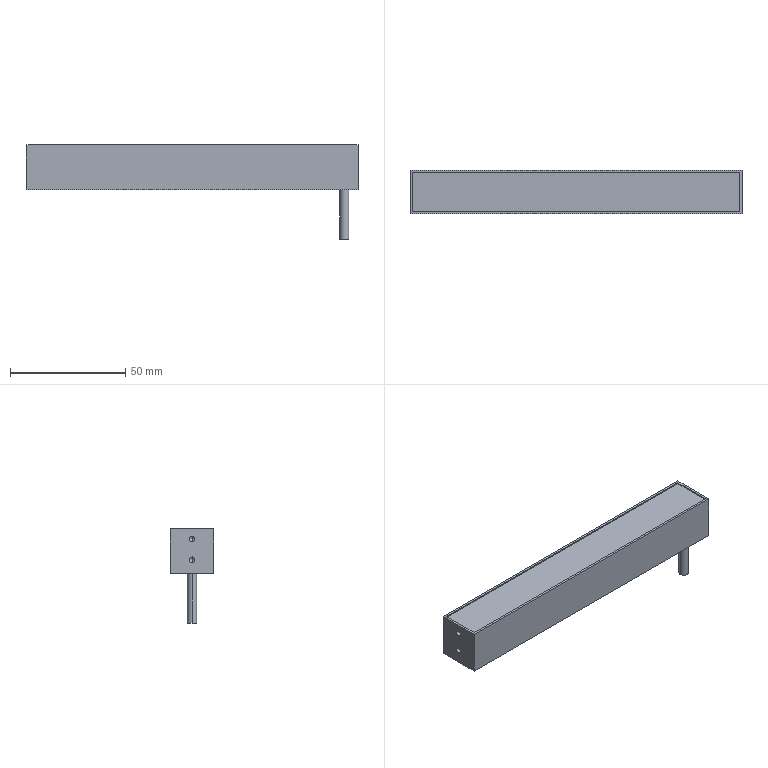Part | STEP file | 11-DHJ-LR-144X1911 | 1 solid | 52 faces | box 144 x 19 x 41 mm | volume 51924 mm3 | plane 26 | cylinder 14 | cone 12 | commonest cylinder face diameters 2.5 x12 4 x2
STEP:
#1=CARTESIAN_POINT('',(43.25,0.,7.5));
#2=VERTEX_POINT('',#1);
#3=CARTESIAN_POINT('',(40.75,0.,7.5));
#4=VERTEX_POINT('',#3);
#5=CARTESIAN_POINT('',(42.,0.,7.5));
#6=DIRECTION('',(0.,0.,-1.));
#7=DIRECTION('',(-1.,0.,0.));
#8=AXIS2_PLACEMENT_3D('',#5,#6,#7);
#9=CIRCLE('',#8,1.25);
#10=EDGE_CURVE('',#2,#4,#9,.T.);
#11=ORIENTED_EDGE('',*,*,#10,.F.);
#12=CARTESIAN_POINT('',(43.25,0.,5.));
#13=VERTEX_POINT('',#12);
#14=CARTESIAN_POINT('',(43.25,0.,0.));
#15=DIRECTION('',(0.,0.,-1.));
#16=VECTOR('',#15,1000.);
#17=LINE('',#14,#16);
#18=EDGE_CURVE('',#2,#13,#17,.T.);
#19=ORIENTED_EDGE('',*,*,#18,.T.);
#20=CARTESIAN_POINT('',(40.75,0.,5.));
#21=VERTEX_POINT('',#20);
#22=CARTESIAN_POINT('',(42.,0.,5.));
#23=DIRECTION('',(0.,0.,-1.));
#24=DIRECTION('',(-1.,0.,0.));
#25=AXIS2_PLACEMENT_3D('',#22,#23,#24);
#26=CIRCLE('',#25,1.25);
#27=EDGE_CURVE('',#13,#21,#26,.T.);
#28=ORIENTED_EDGE('',*,*,#27,.T.);
#29=CARTESIAN_POINT('',(40.75,0.,0.));
#30=DIRECTION('',(0.,0.,-1.));
#31=VECTOR('',#30,1000.);
#32=LINE('',#29,#31);
#33=EDGE_CURVE('',#4,#21,#32,.T.);
#34=ORIENTED_EDGE('',*,*,#33,.F.);
#35=EDGE_LOOP('',(#11,#19,#28,#34));
#36=FACE_OUTER_BOUND('',#35,.T.);
#37=CARTESIAN_POINT('',(42.,0.,0.));
#38=DIRECTION('',(0.,0.,-1.));
#39=DIRECTION('',(-1.,0.,0.));
#40=AXIS2_PLACEMENT_3D('',#37,#38,#39);
#41=CYLINDRICAL_SURFACE('',#40,1.25);
#42=ADVANCED_FACE('',(#36),#41,.F.);
#43=CARTESIAN_POINT('',(42.,0.,8.251));
#44=VERTEX_POINT('',#43);
#45=CARTESIAN_POINT('',(40.75,0.,7.5));
#46=DIRECTION('',(-0.8572,0.,-0.515));
#47=VECTOR('',#46,1000.);
#48=LINE('',#45,#47);
#49=EDGE_CURVE('',#44,#4,#48,.T.);
#50=ORIENTED_EDGE('',*,*,#49,.F.);
#51=CARTESIAN_POINT('',(43.25,0.,7.5));
#52=DIRECTION('',(0.8572,0.,-0.515));
#53=VECTOR('',#52,1000.);
#54=LINE('',#51,#53);
#55=EDGE_CURVE('',#44,#2,#54,.T.);
#56=ORIENTED_EDGE('',*,*,#55,.T.);
#57=ORIENTED_EDGE('',*,*,#10,.T.);
#58=EDGE_LOOP('',(#50,#56,#57));
#59=FACE_OUTER_BOUND('',#58,.T.);
#60=CARTESIAN_POINT('',(42.,0.,7.5));
#61=DIRECTION('',(0.,0.,-1.));
#62=DIRECTION('',(-1.,0.,0.));
#63=AXIS2_PLACEMENT_3D('',#60,#61,#62);
#64=CONICAL_SURFACE('',#63,1.25,1.03);
#65=ADVANCED_FACE('',(#59),#64,.F.);
#66=CARTESIAN_POINT('',(-40.75,0.,7.5));
#67=VERTEX_POINT('',#66);
#68=CARTESIAN_POINT('',(-43.25,0.,7.5));
#69=VERTEX_POINT('',#68);
#70=CARTESIAN_POINT('',(-42.,0.,7.5));
#71=DIRECTION('',(0.,0.,-1.));
#72=DIRECTION('',(-1.,0.,0.));
#73=AXIS2_PLACEMENT_3D('',#70,#71,#72);
#74=CIRCLE('',#73,1.25);
#75=EDGE_CURVE('',#67,#69,#74,.T.);
#76=ORIENTED_EDGE('',*,*,#75,.F.);
#77=CARTESIAN_POINT('',(-40.75,0.,5.));
#78=VERTEX_POINT('',#77);
#79=CARTESIAN_POINT('',(-40.75,0.,0.));
#80=DIRECTION('',(0.,0.,-1.));
#81=VECTOR('',#80,1000.);
#82=LINE('',#79,#81);
#83=EDGE_CURVE('',#67,#78,#82,.T.);
#84=ORIENTED_EDGE('',*,*,#83,.T.);
#85=CARTESIAN_POINT('',(-43.25,0.,5.));
#86=VERTEX_POINT('',#85);
#87=CARTESIAN_POINT('',(-42.,0.,5.));
#88=DIRECTION('',(0.,0.,-1.));
#89=DIRECTION('',(-1.,0.,0.));
#90=AXIS2_PLACEMENT_3D('',#87,#88,#89);
#91=CIRCLE('',#90,1.25);
#92=EDGE_CURVE('',#78,#86,#91,.T.);
#93=ORIENTED_EDGE('',*,*,#92,.T.);
#94=CARTESIAN_POINT('',(-43.25,0.,0.));
#95=DIRECTION('',(0.,0.,-1.));
#96=VECTOR('',#95,1000.);
#97=LINE('',#94,#96);
#98=EDGE_CURVE('',#69,#86,#97,.T.);
#99=ORIENTED_EDGE('',*,*,#98,.F.);
#100=EDGE_LOOP('',(#76,#84,#93,#99));
#101=FACE_OUTER_BOUND('',#100,.T.);
#102=CARTESIAN_POINT('',(-42.,0.,0.));
#103=DIRECTION('',(0.,0.,-1.));
#104=DIRECTION('',(-1.,0.,0.));
#105=AXIS2_PLACEMENT_3D('',#102,#103,#104);
#106=CYLINDRICAL_SURFACE('',#105,1.25);
#107=ADVANCED_FACE('',(#101),#106,.F.);
#108=CARTESIAN_POINT('',(-42.,0.,8.251));
#109=VERTEX_POINT('',#108);
#110=CARTESIAN_POINT('',(-43.25,0.,7.5));
#111=DIRECTION('',(-0.8572,0.,-0.515));
#112=VECTOR('',#111,1000.);
#113=LINE('',#110,#112);
#114=EDGE_CURVE('',#109,#69,#113,.T.);
#115=ORIENTED_EDGE('',*,*,#114,.F.);
#116=CARTESIAN_POINT('',(-40.75,0.,7.5));
#117=DIRECTION('',(0.8572,0.,-0.515));
#118=VECTOR('',#117,1000.);
#119=LINE('',#116,#118);
#120=EDGE_CURVE('',#109,#67,#119,.T.);
#121=ORIENTED_EDGE('',*,*,#120,.T.);
#122=ORIENTED_EDGE('',*,*,#75,.T.);
#123=EDGE_LOOP('',(#115,#121,#122));
#124=FACE_OUTER_BOUND('',#123,.T.);
#125=CARTESIAN_POINT('',(-42.,0.,7.5));
#126=DIRECTION('',(0.,0.,-1.));
#127=DIRECTION('',(-1.,0.,0.));
#128=AXIS2_PLACEMENT_3D('',#125,#126,#127);
#129=CONICAL_SURFACE('',#128,1.25,1.03);
#130=ADVANCED_FACE('',(#124),#129,.F.);
#131=CARTESIAN_POINT('',(64.,0.,-21.5));
#132=VERTEX_POINT('',#131);
#133=CARTESIAN_POINT('',(68.,0.,-21.5));
#134=VERTEX_POINT('',#133);
#135=CARTESIAN_POINT('',(66.,0.,-21.5));
#136=DIRECTION('',(0.,0.,-1.));
#137=DIRECTION('',(-1.,0.,0.));
#138=AXIS2_PLACEMENT_3D('',#135,#136,#137);
#139=CIRCLE('',#138,2.);
#140=EDGE_CURVE('',#132,#134,#139,.T.);
#141=ORIENTED_EDGE('',*,*,#140,.F.);
#142=CARTESIAN_POINT('',(64.,0.,0.));
#143=VERTEX_POINT('',#142);
#144=CARTESIAN_POINT('',(64.,0.,-21.5));
#145=DIRECTION('',(0.,0.,1.));
#146=VECTOR('',#145,1000.);
#147=LINE('',#144,#146);
#148=EDGE_CURVE('',#132,#143,#147,.T.);
#149=ORIENTED_EDGE('',*,*,#148,.T.);
#150=CARTESIAN_POINT('',(68.,0.,0.));
#151=VERTEX_POINT('',#150);
#152=CARTESIAN_POINT('',(66.,0.,0.));
#153=DIRECTION('',(0.,0.,-1.));
#154=DIRECTION('',(1.,0.,0.));
#155=AXIS2_PLACEMENT_3D('',#152,#153,#154);
#156=CIRCLE('',#155,2.);
#157=EDGE_CURVE('',#143,#151,#156,.T.);
#158=ORIENTED_EDGE('',*,*,#157,.T.);
#159=CARTESIAN_POINT('',(68.,0.,-21.5));
#160=DIRECTION('',(0.,0.,1.));
#161=VECTOR('',#160,1000.);
#162=LINE('',#159,#161);
#163=EDGE_CURVE('',#134,#151,#162,.T.);
#164=ORIENTED_EDGE('',*,*,#163,.F.);
#165=EDGE_LOOP('',(#141,#149,#158,#164));
#166=FACE_OUTER_BOUND('',#165,.T.);
#167=CARTESIAN_POINT('',(66.,0.,-21.5));
#168=DIRECTION('',(0.,0.,1.));
#169=DIRECTION('',(1.,0.,0.));
#170=AXIS2_PLACEMENT_3D('',#167,#168,#169);
#171=CYLINDRICAL_SURFACE('',#170,2.);
#172=ADVANCED_FACE('',(#166),#171,.T.);
#173=CARTESIAN_POINT('',(-64.5,0.,4.75));
#174=VERTEX_POINT('',#173);
#175=CARTESIAN_POINT('',(-64.5,0.,7.25));
#176=VERTEX_POINT('',#175);
#177=CARTESIAN_POINT('',(-64.5,0.,6.));
#178=DIRECTION('',(-1.,0.,0.));
#179=DIRECTION('',(0.,0.,1.));
#180=AXIS2_PLACEMENT_3D('',#177,#178,#179);
#181=CIRCLE('',#180,1.25);
#182=EDGE_CURVE('',#174,#176,#181,.T.);
#183=ORIENTED_EDGE('',*,*,#182,.F.);
#184=CARTESIAN_POINT('',(-72.,0.,4.75));
#185=VERTEX_POINT('',#184);
#186=CARTESIAN_POINT('',(-72.,0.,4.75));
#187=DIRECTION('',(-1.,0.,0.));
#188=VECTOR('',#187,1000.);
#189=LINE('',#186,#188);
#190=EDGE_CURVE('',#174,#185,#189,.T.);
#191=ORIENTED_EDGE('',*,*,#190,.T.);
#192=CARTESIAN_POINT('',(-72.,0.,7.25));
#193=VERTEX_POINT('',#192);
#194=CARTESIAN_POINT('',(-72.,0.,6.));
#195=DIRECTION('',(-1.,0.,0.));
#196=DIRECTION('',(0.,0.,1.));
#197=AXIS2_PLACEMENT_3D('',#194,#195,#196);
#198=CIRCLE('',#197,1.25);
#199=EDGE_CURVE('',#185,#193,#198,.T.);
#200=ORIENTED_EDGE('',*,*,#199,.T.);
#201=CARTESIAN_POINT('',(-72.,0.,7.25));
#202=DIRECTION('',(-1.,0.,0.));
#203=VECTOR('',#202,1000.);
#204=LINE('',#201,#203);
#205=EDGE_CURVE('',#176,#193,#204,.T.);
#206=ORIENTED_EDGE('',*,*,#205,.F.);
#207=EDGE_LOOP('',(#183,#191,#200,#206));
#208=FACE_OUTER_BOUND('',#207,.T.);
#209=CARTESIAN_POINT('',(-72.,0.,6.));
#210=DIRECTION('',(-1.,0.,0.));
#211=DIRECTION('',(0.,0.,1.));
#212=AXIS2_PLACEMENT_3D('',#209,#210,#211);
#213=CYLINDRICAL_SURFACE('',#212,1.25);
#214=ADVANCED_FACE('',(#208),#213,.F.);
#215=CARTESIAN_POINT('',(-63.749,0.,6.));
#216=VERTEX_POINT('',#215);
#217=CARTESIAN_POINT('',(-64.5,0.,7.25));
#218=DIRECTION('',(-0.515,0.,0.8572));
#219=VECTOR('',#218,1000.);
#220=LINE('',#217,#219);
#221=EDGE_CURVE('',#216,#176,#220,.T.);
#222=ORIENTED_EDGE('',*,*,#221,.F.);
#223=CARTESIAN_POINT('',(-64.5,0.,4.75));
#224=DIRECTION('',(-0.515,0.,-0.8572));
#225=VECTOR('',#224,1000.);
#226=LINE('',#223,#225);
#227=EDGE_CURVE('',#216,#174,#226,.T.);
#228=ORIENTED_EDGE('',*,*,#227,.T.);
#229=ORIENTED_EDGE('',*,*,#182,.T.);
#230=EDGE_LOOP('',(#222,#228,#229));
#231=FACE_OUTER_BOUND('',#230,.T.);
#232=CARTESIAN_POINT('',(-64.5,0.,6.));
#233=DIRECTION('',(-1.,0.,0.));
#234=DIRECTION('',(0.,0.,1.));
#235=AXIS2_PLACEMENT_3D('',#232,#233,#234);
#236=CONICAL_SURFACE('',#235,1.25,1.03);
#237=ADVANCED_FACE('',(#231),#236,.F.);
#238=CARTESIAN_POINT('',(-64.5,0.,13.75));
#239=VERTEX_POINT('',#238);
#240=CARTESIAN_POINT('',(-64.5,0.,16.25));
#241=VERTEX_POINT('',#240);
#242=CARTESIAN_POINT('',(-64.5,0.,15.));
#243=DIRECTION('',(-1.,0.,0.));
#244=DIRECTION('',(0.,0.,1.));
#245=AXIS2_PLACEMENT_3D('',#242,#243,#244);
#246=CIRCLE('',#245,1.25);
#247=EDGE_CURVE('',#239,#241,#246,.T.);
#248=ORIENTED_EDGE('',*,*,#247,.F.);
#249=CARTESIAN_POINT('',(-72.,0.,13.75));
#250=VERTEX_POINT('',#249);
#251=CARTESIAN_POINT('',(-72.,0.,13.75));
#252=DIRECTION('',(-1.,0.,0.));
#253=VECTOR('',#252,1000.);
#254=LINE('',#251,#253);
#255=EDGE_CURVE('',#239,#250,#254,.T.);
#256=ORIENTED_EDGE('',*,*,#255,.T.);
#257=CARTESIAN_POINT('',(-72.,0.,16.25));
#258=VERTEX_POINT('',#257);
#259=CARTESIAN_POINT('',(-72.,0.,15.));
#260=DIRECTION('',(-1.,0.,0.));
#261=DIRECTION('',(0.,0.,1.));
#262=AXIS2_PLACEMENT_3D('',#259,#260,#261);
#263=CIRCLE('',#262,1.25);
#264=EDGE_CURVE('',#250,#258,#263,.T.);
#265=ORIENTED_EDGE('',*,*,#264,.T.);
#266=CARTESIAN_POINT('',(-72.,0.,16.25));
#267=DIRECTION('',(-1.,0.,0.));
#268=VECTOR('',#267,1000.);
#269=LINE('',#266,#268);
#270=EDGE_CURVE('',#241,#258,#269,.T.);
#271=ORIENTED_EDGE('',*,*,#270,.F.);
#272=EDGE_LOOP('',(#248,#256,#265,#271));
#273=FACE_OUTER_BOUND('',#272,.T.);
#274=CARTESIAN_POINT('',(-72.,0.,15.));
#275=DIRECTION('',(-1.,0.,0.));
#276=DIRECTION('',(0.,0.,1.));
#277=AXIS2_PLACEMENT_3D('',#274,#275,#276);
#278=CYLINDRICAL_SURFACE('',#277,1.25);
#279=ADVANCED_FACE('',(#273),#278,.F.);
#280=CARTESIAN_POINT('',(-63.749,0.,15.));
#281=VERTEX_POINT('',#280);
#282=CARTESIAN_POINT('',(-64.5,0.,16.25));
#283=DIRECTION('',(-0.515,0.,0.8572));
#284=VECTOR('',#283,1000.);
#285=LINE('',#282,#284);
#286=EDGE_CURVE('',#281,#241,#285,.T.);
#287=ORIENTED_EDGE('',*,*,#286,.F.);
#288=CARTESIAN_POINT('',(-64.5,0.,13.75));
#289=DIRECTION('',(-0.515,0.,-0.8572));
#290=VECTOR('',#289,1000.);
#291=LINE('',#288,#290);
#292=EDGE_CURVE('',#281,#239,#291,.T.);
#293=ORIENTED_EDGE('',*,*,#292,.T.);
#294=ORIENTED_EDGE('',*,*,#247,.T.);
#295=EDGE_LOOP('',(#287,#293,#294));
#296=FACE_OUTER_BOUND('',#295,.T.);
#297=CARTESIAN_POINT('',(-64.5,0.,15.));
#298=DIRECTION('',(-1.,0.,0.));
#299=DIRECTION('',(0.,0.,1.));
#300=AXIS2_PLACEMENT_3D('',#297,#298,#299);
#301=CONICAL_SURFACE('',#300,1.25,1.03);
#302=ADVANCED_FACE('',(#296),#301,.F.);
#303=CARTESIAN_POINT('',(64.5,0.,16.25));
#304=VERTEX_POINT('',#303);
#305=CARTESIAN_POINT('',(64.5,0.,13.75));
#306=VERTEX_POINT('',#305);
#307=CARTESIAN_POINT('',(64.5,0.,15.));
#308=DIRECTION('',(1.,0.,0.));
#309=DIRECTION('',(0.,0.,-1.));
#310=AXIS2_PLACEMENT_3D('',#307,#308,#309);
#311=CIRCLE('',#310,1.25);
#312=EDGE_CURVE('',#304,#306,#311,.T.);
#313=ORIENTED_EDGE('',*,*,#312,.F.);
#314=CARTESIAN_POINT('',(72.,0.,16.25));
#315=VERTEX_POINT('',#314);
#316=CARTESIAN_POINT('',(72.,0.,16.25));
#317=DIRECTION('',(1.,0.,0.));
#318=VECTOR('',#317,1000.);
#319=LINE('',#316,#318);
#320=EDGE_CURVE('',#304,#315,#319,.T.);
#321=ORIENTED_EDGE('',*,*,#320,.T.);
#322=CARTESIAN_POINT('',(72.,0.,13.75));
#323=VERTEX_POINT('',#322);
#324=CARTESIAN_POINT('',(72.,0.,15.));
#325=DIRECTION('',(1.,0.,0.));
#326=DIRECTION('',(0.,0.,-1.));
#327=AXIS2_PLACEMENT_3D('',#324,#325,#326);
#328=CIRCLE('',#327,1.25);
#329=EDGE_CURVE('',#315,#323,#328,.T.);
#330=ORIENTED_EDGE('',*,*,#329,.T.);
#331=CARTESIAN_POINT('',(72.,0.,13.75));
#332=DIRECTION('',(1.,0.,0.));
#333=VECTOR('',#332,1000.);
#334=LINE('',#331,#333);
#335=EDGE_CURVE('',#306,#323,#334,.T.);
#336=ORIENTED_EDGE('',*,*,#335,.F.);
#337=EDGE_LOOP('',(#313,#321,#330,#336));
#338=FACE_OUTER_BOUND('',#337,.T.);
#339=CARTESIAN_POINT('',(72.,0.,15.));
#340=DIRECTION('',(1.,0.,0.));
#341=DIRECTION('',(0.,0.,-1.));
#342=AXIS2_PLACEMENT_3D('',#339,#340,#341);
#343=CYLINDRICAL_SURFACE('',#342,1.25);
#344=ADVANCED_FACE('',(#338),#343,.F.);
#345=CARTESIAN_POINT('',(63.749,0.,15.));
#346=VERTEX_POINT('',#345);
#347=CARTESIAN_POINT('',(64.5,0.,13.75));
#348=DIRECTION('',(0.515,0.,-0.8572));
#349=VECTOR('',#348,1000.);
#350=LINE('',#347,#349);
#351=EDGE_CURVE('',#346,#306,#350,.T.);
#352=ORIENTED_EDGE('',*,*,#351,.F.);
#353=CARTESIAN_POINT('',(64.5,0.,16.25));
#354=DIRECTION('',(0.515,0.,0.8572));
#355=VECTOR('',#354,1000.);
#356=LINE('',#353,#355);
#357=EDGE_CURVE('',#346,#304,#356,.T.);
#358=ORIENTED_EDGE('',*,*,#357,.T.);
#359=ORIENTED_EDGE('',*,*,#312,.T.);
#360=EDGE_LOOP('',(#352,#358,#359));
#361=FACE_OUTER_BOUND('',#360,.T.);
#362=CARTESIAN_POINT('',(64.5,0.,15.));
#363=DIRECTION('',(1.,0.,0.));
#364=DIRECTION('',(0.,0.,-1.));
#365=AXIS2_PLACEMENT_3D('',#362,#363,#364);
#366=CONICAL_SURFACE('',#365,1.25,1.03);
#367=ADVANCED_FACE('',(#361),#366,.F.);
#368=CARTESIAN_POINT('',(64.5,0.,7.25));
#369=VERTEX_POINT('',#368);
#370=CARTESIAN_POINT('',(64.5,0.,4.75));
#371=VERTEX_POINT('',#370);
#372=CARTESIAN_POINT('',(64.5,0.,6.));
#373=DIRECTION('',(1.,0.,0.));
#374=DIRECTION('',(0.,0.,-1.));
#375=AXIS2_PLACEMENT_3D('',#372,#373,#374);
#376=CIRCLE('',#375,1.25);
#377=EDGE_CURVE('',#369,#371,#376,.T.);
#378=ORIENTED_EDGE('',*,*,#377,.F.);
#379=CARTESIAN_POINT('',(72.,0.,7.25));
#380=VERTEX_POINT('',#379);
#381=CARTESIAN_POINT('',(72.,0.,7.25));
#382=DIRECTION('',(1.,0.,0.));
#383=VECTOR('',#382,1000.);
#384=LINE('',#381,#383);
#385=EDGE_CURVE('',#369,#380,#384,.T.);
#386=ORIENTED_EDGE('',*,*,#385,.T.);
#387=CARTESIAN_POINT('',(72.,0.,4.75));
#388=VERTEX_POINT('',#387);
#389=CARTESIAN_POINT('',(72.,0.,6.));
#390=DIRECTION('',(1.,0.,0.));
#391=DIRECTION('',(0.,0.,-1.));
#392=AXIS2_PLACEMENT_3D('',#389,#390,#391);
#393=CIRCLE('',#392,1.25);
#394=EDGE_CURVE('',#380,#388,#393,.T.);
#395=ORIENTED_EDGE('',*,*,#394,.T.);
#396=CARTESIAN_POINT('',(72.,0.,4.75));
#397=DIRECTION('',(1.,0.,0.));
#398=VECTOR('',#397,1000.);
#399=LINE('',#396,#398);
#400=EDGE_CURVE('',#371,#388,#399,.T.);
#401=ORIENTED_EDGE('',*,*,#400,.F.);
#402=EDGE_LOOP('',(#378,#386,#395,#401));
#403=FACE_OUTER_BOUND('',#402,.T.);
#404=CARTESIAN_POINT('',(72.,0.,6.));
#405=DIRECTION('',(1.,0.,0.));
#406=DIRECTION('',(0.,0.,-1.));
#407=AXIS2_PLACEMENT_3D('',#404,#405,#406);
#408=CYLINDRICAL_SURFACE('',#407,1.25);
#409=ADVANCED_FACE('',(#403),#408,.F.);
#410=CARTESIAN_POINT('',(63.749,0.,6.));
#411=VERTEX_POINT('',#410);
#412=CARTESIAN_POINT('',(64.5,0.,4.75));
#413=DIRECTION('',(0.515,0.,-0.8572));
#414=VECTOR('',#413,1000.);
#415=LINE('',#412,#414);
#416=EDGE_CURVE('',#411,#371,#415,.T.);
#417=ORIENTED_EDGE('',*,*,#416,.F.);
#418=CARTESIAN_POINT('',(64.5,0.,7.25));
#419=DIRECTION('',(0.515,0.,0.8572));
#420=VECTOR('',#419,1000.);
#421=LINE('',#418,#420);
#422=EDGE_CURVE('',#411,#369,#421,.T.);
#423=ORIENTED_EDGE('',*,*,#422,.T.);
#424=ORIENTED_EDGE('',*,*,#377,.T.);
#425=EDGE_LOOP('',(#417,#423,#424));
#426=FACE_OUTER_BOUND('',#425,.T.);
#427=CARTESIAN_POINT('',(64.5,0.,6.));
#428=DIRECTION('',(1.,0.,0.));
#429=DIRECTION('',(0.,0.,-1.));
#430=AXIS2_PLACEMENT_3D('',#427,#428,#429);
#431=CONICAL_SURFACE('',#430,1.25,1.03);
#432=ADVANCED_FACE('',(#426),#431,.F.);
#433=CARTESIAN_POINT('',(72.,0.,15.));
#434=DIRECTION('',(1.,0.,0.));
#435=DIRECTION('',(0.,0.,-1.));
#436=AXIS2_PLACEMENT_3D('',#433,#434,#435);
#437=CIRCLE('',#436,1.25);
#438=EDGE_CURVE('',#323,#315,#437,.T.);
#439=ORIENTED_EDGE('',*,*,#438,.F.);
#440=ORIENTED_EDGE('',*,*,#329,.F.);
#441=EDGE_LOOP('',(#439,#440));
#442=FACE_BOUND('',#441,.T.);
#443=CARTESIAN_POINT('',(72.,0.,6.));
#444=DIRECTION('',(1.,0.,0.));
#445=DIRECTION('',(0.,0.,-1.));
#446=AXIS2_PLACEMENT_3D('',#443,#444,#445);
#447=CIRCLE('',#446,1.25);
#448=EDGE_CURVE('',#388,#380,#447,.T.);
#449=ORIENTED_EDGE('',*,*,#448,.F.);
#450=ORIENTED_EDGE('',*,*,#394,.F.);
#451=EDGE_LOOP('',(#449,#450));
#452=FACE_BOUND('',#451,.T.);
#453=CARTESIAN_POINT('',(72.,-9.5,0.));
#454=VERTEX_POINT('',#453);
#455=CARTESIAN_POINT('',(72.,9.5,0.));
#456=VERTEX_POINT('',#455);
#457=CARTESIAN_POINT('',(72.,9.5,0.));
#458=DIRECTION('',(0.,1.,0.));
#459=VECTOR('',#458,1000.);
#460=LINE('',#457,#459);
#461=EDGE_CURVE('',#454,#456,#460,.T.);
#462=ORIENTED_EDGE('',*,*,#461,.T.);
#463=CARTESIAN_POINT('',(72.,9.5,19.5));
#464=VERTEX_POINT('',#463);
#465=CARTESIAN_POINT('',(72.,9.5,19.5));
#466=DIRECTION('',(0.,0.,-1.));
#467=VECTOR('',#466,1000.);
#468=LINE('',#465,#467);
#469=EDGE_CURVE('',#464,#456,#468,.T.);
#470=ORIENTED_EDGE('',*,*,#469,.F.);
#471=CARTESIAN_POINT('',(72.,-9.5,19.5));
#472=VERTEX_POINT('',#471);
#473=CARTESIAN_POINT('',(72.,9.5,19.5));
#474=DIRECTION('',(0.,1.,0.));
#475=VECTOR('',#474,1000.);
#476=LINE('',#473,#475);
#477=EDGE_CURVE('',#472,#464,#476,.T.);
#478=ORIENTED_EDGE('',*,*,#477,.F.);
#479=CARTESIAN_POINT('',(72.,-9.5,19.5));
#480=DIRECTION('',(0.,0.,-1.));
#481=VECTOR('',#480,1000.);
#482=LINE('',#479,#481);
#483=EDGE_CURVE('',#472,#454,#482,.T.);
#484=ORIENTED_EDGE('',*,*,#483,.T.);
#485=EDGE_LOOP('',(#462,#470,#478,#484));
#486=FACE_OUTER_BOUND('',#485,.T.);
#487=CARTESIAN_POINT('',(72.,9.5,19.5));
#488=DIRECTION('',(-1.,0.,0.));
#489=DIRECTION('',(0.,0.,1.));
#490=AXIS2_PLACEMENT_3D('',#487,#488,#489);
#491=PLANE('',#490);
#492=ADVANCED_FACE('',(#442,#452,#486),#491,.F.);
#493=CARTESIAN_POINT('',(-72.,9.5,0.));
#494=VERTEX_POINT('',#493);
#495=CARTESIAN_POINT('',(-72.,9.5,0.));
#496=DIRECTION('',(-1.,0.,0.));
#497=VECTOR('',#496,1000.);
#498=LINE('',#495,#497);
#499=EDGE_CURVE('',#456,#494,#498,.T.);
#500=ORIENTED_EDGE('',*,*,#499,.T.);
#501=CARTESIAN_POINT('',(-72.,9.5,19.5));
#502=VERTEX_POINT('',#501);
#503=CARTESIAN_POINT('',(-72.,9.5,19.5));
#504=DIRECTION('',(0.,0.,-1.));
#505=VECTOR('',#504,1000.);
#506=LINE('',#503,#505);
#507=EDGE_CURVE('',#502,#494,#506,.T.);
#508=ORIENTED_EDGE('',*,*,#507,.F.);
#509=CARTESIAN_POINT('',(-72.,9.5,19.5));
#510=DIRECTION('',(-1.,0.,0.));
#511=VECTOR('',#510,1000.);
#512=LINE('',#509,#511);
#513=EDGE_CURVE('',#464,#502,#512,.T.);
#514=ORIENTED_EDGE('',*,*,#513,.F.);
#515=ORIENTED_EDGE('',*,*,#469,.T.);
#516=EDGE_LOOP('',(#500,#508,#514,#515));
#517=FACE_OUTER_BOUND('',#516,.T.);
#518=CARTESIAN_POINT('',(-72.,9.5,19.5));
#519=DIRECTION('',(0.,-1.,0.));
#520=DIRECTION('',(0.,0.,-1.));
#521=AXIS2_PLACEMENT_3D('',#518,#519,#520);
#522=PLANE('',#521);
#523=ADVANCED_FACE('',(#517),#522,.F.);
#524=CARTESIAN_POINT('',(-72.,0.,6.));
#525=DIRECTION('',(-1.,0.,0.));
#526=DIRECTION('',(0.,0.,1.));
#527=AXIS2_PLACEMENT_3D('',#524,#525,#526);
#528=CIRCLE('',#527,1.25);
#529=EDGE_CURVE('',#193,#185,#528,.T.);
#530=ORIENTED_EDGE('',*,*,#529,.F.);
#531=ORIENTED_EDGE('',*,*,#199,.F.);
#532=EDGE_LOOP('',(#530,#531));
#533=FACE_BOUND('',#532,.T.);
#534=CARTESIAN_POINT('',(-72.,0.,15.));
#535=DIRECTION('',(-1.,0.,0.));
#536=DIRECTION('',(0.,0.,1.));
#537=AXIS2_PLACEMENT_3D('',#534,#535,#536);
#538=CIRCLE('',#537,1.25);
#539=EDGE_CURVE('',#258,#250,#538,.T.);
#540=ORIENTED_EDGE('',*,*,#539,.F.);
#541=ORIENTED_EDGE('',*,*,#264,.F.);
#542=EDGE_LOOP('',(#540,#541));
#543=FACE_BOUND('',#542,.T.);
#544=CARTESIAN_POINT('',(-72.,-9.5,0.));
#545=VERTEX_POINT('',#544);
#546=CARTESIAN_POINT('',(-72.,9.5,0.));
#547=DIRECTION('',(0.,-1.,0.));
#548=VECTOR('',#547,1000.);
#549=LINE('',#546,#548);
#550=EDGE_CURVE('',#494,#545,#549,.T.);
#551=ORIENTED_EDGE('',*,*,#550,.T.);
#552=CARTESIAN_POINT('',(-72.,-9.5,19.5));
#553=VERTEX_POINT('',#552);
#554=CARTESIAN_POINT('',(-72.,-9.5,19.5));
#555=DIRECTION('',(0.,0.,-1.));
#556=VECTOR('',#555,1000.);
#557=LINE('',#554,#556);
#558=EDGE_CURVE('',#553,#545,#557,.T.);
#559=ORIENTED_EDGE('',*,*,#558,.F.);
#560=CARTESIAN_POINT('',(-72.,9.5,19.5));
#561=DIRECTION('',(0.,-1.,0.));
#562=VECTOR('',#561,1000.);
#563=LINE('',#560,#562);
#564=EDGE_CURVE('',#502,#553,#563,.T.);
#565=ORIENTED_EDGE('',*,*,#564,.F.);
#566=ORIENTED_EDGE('',*,*,#507,.T.);
#567=EDGE_LOOP('',(#551,#559,#565,#566));
#568=FACE_OUTER_BOUND('',#567,.T.);
#569=CARTESIAN_POINT('',(-72.,9.5,19.5));
#570=DIRECTION('',(1.,0.,0.));
#571=DIRECTION('',(0.,0.,-1.));
#572=AXIS2_PLACEMENT_3D('',#569,#570,#571);
#573=PLANE('',#572);
#574=ADVANCED_FACE('',(#533,#543,#568),#573,.F.);
#575=CARTESIAN_POINT('',(-72.,-9.5,0.));
#576=DIRECTION('',(1.,0.,0.));
#577=VECTOR('',#576,1000.);
#578=LINE('',#575,#577);
#579=EDGE_CURVE('',#545,#454,#578,.T.);
#580=ORIENTED_EDGE('',*,*,#579,.T.);
#581=ORIENTED_EDGE('',*,*,#483,.F.);
#582=CARTESIAN_POINT('',(-72.,-9.5,19.5));
#583=DIRECTION('',(1.,0.,0.));
#584=VECTOR('',#583,1000.);
#585=LINE('',#582,#584);
#586=EDGE_CURVE('',#553,#472,#585,.T.);
#587=ORIENTED_EDGE('',*,*,#586,.F.);
#588=ORIENTED_EDGE('',*,*,#558,.T.);
#589=EDGE_LOOP('',(#580,#581,#587,#588));
#590=FACE_OUTER_BOUND('',#589,.T.);
#591=CARTESIAN_POINT('',(-72.,-9.5,19.5));
#592=DIRECTION('',(0.,1.,0.));
#593=DIRECTION('',(0.,0.,1.));
#594=AXIS2_PLACEMENT_3D('',#591,#592,#593);
#595=PLANE('',#594);
#596=ADVANCED_FACE('',(#590),#595,.F.);
#597=CARTESIAN_POINT('',(71.,-8.5,19.5));
#598=VERTEX_POINT('',#597);
#599=CARTESIAN_POINT('',(71.,8.5,19.5));
#600=VERTEX_POINT('',#599);
#601=CARTESIAN_POINT('',(71.,-8.5,19.5));
#602=DIRECTION('',(0.,1.,0.));
#603=VECTOR('',#602,1000.);
#604=LINE('',#601,#603);
#605=EDGE_CURVE('',#598,#600,#604,.T.);
#606=ORIENTED_EDGE('',*,*,#605,.F.);
#607=CARTESIAN_POINT('',(-71.,-8.5,19.5));
#608=VERTEX_POINT('',#607);
#609=CARTESIAN_POINT('',(-71.,-8.5,19.5));
#610=DIRECTION('',(1.,0.,0.));
#611=VECTOR('',#610,1000.);
#612=LINE('',#609,#611);
#613=EDGE_CURVE('',#608,#598,#612,.T.);
#614=ORIENTED_EDGE('',*,*,#613,.F.);
#615=CARTESIAN_POINT('',(-71.,8.5,19.5));
#616=VERTEX_POINT('',#615);
#617=CARTESIAN_POINT('',(-71.,-8.5,19.5));
#618=DIRECTION('',(0.,-1.,0.));
#619=VECTOR('',#618,1000.);
#620=LINE('',#617,#619);
#621=EDGE_CURVE('',#616,#608,#620,.T.);
#622=ORIENTED_EDGE('',*,*,#621,.F.);
#623=CARTESIAN_POINT('',(-71.,8.5,19.5));
#624=DIRECTION('',(-1.,0.,0.));
#625=VECTOR('',#624,1000.);
#626=LINE('',#623,#625);
#627=EDGE_CURVE('',#600,#616,#626,.T.);
#628=ORIENTED_EDGE('',*,*,#627,.F.);
#629=EDGE_LOOP('',(#606,#614,#622,#628));
#630=FACE_BOUND('',#629,.T.);
#631=ORIENTED_EDGE('',*,*,#477,.T.);
#632=ORIENTED_EDGE('',*,*,#513,.T.);
#633=ORIENTED_EDGE('',*,*,#564,.T.);
#634=ORIENTED_EDGE('',*,*,#586,.T.);
#635=EDGE_LOOP('',(#631,#632,#633,#634));
#636=FACE_OUTER_BOUND('',#635,.T.);
#637=CARTESIAN_POINT('',(0.,0.,19.5));
#638=DIRECTION('',(0.,0.,1.));
#639=DIRECTION('',(1.,0.,0.));
#640=AXIS2_PLACEMENT_3D('',#637,#638,#639);
#641=PLANE('',#640);
#642=ADVANCED_FACE('',(#630,#636),#641,.T.);
#643=CARTESIAN_POINT('',(-45.464,0.,0.));
#644=VERTEX_POINT('',#643);
#645=CARTESIAN_POINT('',(-43.732,3.,0.));
#646=VERTEX_POINT('',#645);
#647=CARTESIAN_POINT('',(-45.464,0.,0.));
#648=DIRECTION('',(0.5,0.866,0.));
#649=VECTOR('',#648,1000.);
#650=LINE('',#647,#649);
#651=EDGE_CURVE('',#644,#646,#650,.T.);
#652=ORIENTED_EDGE('',*,*,#651,.F.);
#653=CARTESIAN_POINT('',(-43.732,-3.,0.));
#654=VERTEX_POINT('',#653);
#655=CARTESIAN_POINT('',(-43.732,-3.,0.));
#656=DIRECTION('',(-0.5,0.866,0.));
#657=VECTOR('',#656,1000.);
#658=LINE('',#655,#657);
#659=EDGE_CURVE('',#654,#644,#658,.T.);
#660=ORIENTED_EDGE('',*,*,#659,.F.);
#661=CARTESIAN_POINT('',(-40.268,-3.,0.));
#662=VERTEX_POINT('',#661);
#663=CARTESIAN_POINT('',(-40.268,-3.,0.));
#664=DIRECTION('',(-1.,0.,0.));
#665=VECTOR('',#664,1000.);
#666=LINE('',#663,#665);
#667=EDGE_CURVE('',#662,#654,#666,.T.);
#668=ORIENTED_EDGE('',*,*,#667,.F.);
#669=CARTESIAN_POINT('',(-38.536,0.,0.));
#670=VERTEX_POINT('',#669);
#671=CARTESIAN_POINT('',(-38.536,0.,0.));
#672=DIRECTION('',(-0.5,-0.866,0.));
#673=VECTOR('',#672,1000.);
#674=LINE('',#671,#673);
#675=EDGE_CURVE('',#670,#662,#674,.T.);
#676=ORIENTED_EDGE('',*,*,#675,.F.);
#677=CARTESIAN_POINT('',(-40.268,3.,0.));
#678=VERTEX_POINT('',#677);
#679=CARTESIAN_POINT('',(-40.268,3.,0.));
#680=DIRECTION('',(0.5,-0.866,0.));
#681=VECTOR('',#680,1000.);
#682=LINE('',#679,#681);
#683=EDGE_CURVE('',#678,#670,#682,.T.);
#684=ORIENTED_EDGE('',*,*,#683,.F.);
#685=CARTESIAN_POINT('',(-43.732,3.,0.));
#686=DIRECTION('',(1.,0.,0.));
#687=VECTOR('',#686,1000.);
#688=LINE('',#685,#687);
#689=EDGE_CURVE('',#646,#678,#688,.T.);
#690=ORIENTED_EDGE('',*,*,#689,.F.);
#691=EDGE_LOOP('',(#652,#660,#668,#676,#684,#690));
#692=FACE_BOUND('',#691,.T.);
#693=CARTESIAN_POINT('',(38.536,0.,0.));
#694=VERTEX_POINT('',#693);
#695=CARTESIAN_POINT('',(40.268,3.,0.));
#696=VERTEX_POINT('',#695);
#697=CARTESIAN_POINT('',(38.536,0.,0.));
#698=DIRECTION('',(0.5,0.866,0.));
#699=VECTOR('',#698,1000.);
#700=LINE('',#697,#699);
#701=EDGE_CURVE('',#694,#696,#700,.T.);
#702=ORIENTED_EDGE('',*,*,#701,.F.);
#703=CARTESIAN_POINT('',(40.268,-3.,0.));
#704=VERTEX_POINT('',#703);
#705=CARTESIAN_POINT('',(40.268,-3.,0.));
#706=DIRECTION('',(-0.5,0.866,0.));
#707=VECTOR('',#706,1000.);
#708=LINE('',#705,#707);
#709=EDGE_CURVE('',#704,#694,#708,.T.);
#710=ORIENTED_EDGE('',*,*,#709,.F.);
#711=CARTESIAN_POINT('',(43.732,-3.,0.));
#712=VERTEX_POINT('',#711);
#713=CARTESIAN_POINT('',(43.732,-3.,0.));
#714=DIRECTION('',(-1.,0.,0.));
#715=VECTOR('',#714,1000.);
#716=LINE('',#713,#715);
#717=EDGE_CURVE('',#712,#704,#716,.T.);
#718=ORIENTED_EDGE('',*,*,#717,.F.);
#719=CARTESIAN_POINT('',(45.464,0.,0.));
#720=VERTEX_POINT('',#719);
#721=CARTESIAN_POINT('',(45.464,0.,0.));
#722=DIRECTION('',(-0.5,-0.866,0.));
#723=VECTOR('',#722,1000.);
#724=LINE('',#721,#723);
#725=EDGE_CURVE('',#720,#712,#724,.T.);
#726=ORIENTED_EDGE('',*,*,#725,.F.);
#727=CARTESIAN_POINT('',(43.732,3.,0.));
#728=VERTEX_POINT('',#727);
#729=CARTESIAN_POINT('',(43.732,3.,0.));
#730=DIRECTION('',(0.5,-0.866,0.));
#731=VECTOR('',#730,1000.);
#732=LINE('',#729,#731);
#733=EDGE_CURVE('',#728,#720,#732,.T.);
#734=ORIENTED_EDGE('',*,*,#733,.F.);
#735=CARTESIAN_POINT('',(40.268,3.,0.));
#736=DIRECTION('',(1.,0.,0.));
#737=VECTOR('',#736,1000.);
#738=LINE('',#735,#737);
#739=EDGE_CURVE('',#696,#728,#738,.T.);
#740=ORIENTED_EDGE('',*,*,#739,.F.);
#741=EDGE_LOOP('',(#702,#710,#718,#726,#734,#740));
#742=FACE_BOUND('',#741,.T.);
#743=CARTESIAN_POINT('',(66.,0.,0.));
#744=DIRECTION('',(0.,0.,-1.));
#745=DIRECTION('',(1.,0.,0.));
#746=AXIS2_PLACEMENT_3D('',#743,#744,#745);
#747=CIRCLE('',#746,2.);
#748=EDGE_CURVE('',#151,#143,#747,.T.);
#749=ORIENTED_EDGE('',*,*,#748,.F.);
#750=ORIENTED_EDGE('',*,*,#157,.F.);
#751=EDGE_LOOP('',(#749,#750));
#752=FACE_BOUND('',#751,.T.);
#753=ORIENTED_EDGE('',*,*,#461,.F.);
#754=ORIENTED_EDGE('',*,*,#579,.F.);
#755=ORIENTED_EDGE('',*,*,#550,.F.);
#756=ORIENTED_EDGE('',*,*,#499,.F.);
#757=EDGE_LOOP('',(#753,#754,#755,#756));
#758=FACE_OUTER_BOUND('',#757,.T.);
#759=CARTESIAN_POINT('',(0.,0.,0.));
#760=DIRECTION('',(0.,0.,1.));
#761=DIRECTION('',(1.,0.,0.));
#762=AXIS2_PLACEMENT_3D('',#759,#760,#761);
#763=PLANE('',#762);
#764=ADVANCED_FACE('',(#692,#742,#752,#758),#763,.F.);
#765=ORIENTED_EDGE('',*,*,#605,.T.);
#766=CARTESIAN_POINT('',(71.,8.5,19.));
#767=VERTEX_POINT('',#766);
#768=CARTESIAN_POINT('',(71.,8.5,19.));
#769=DIRECTION('',(0.,0.,1.));
#770=VECTOR('',#769,1000.);
#771=LINE('',#768,#770);
#772=EDGE_CURVE('',#767,#600,#771,.T.);
#773=ORIENTED_EDGE('',*,*,#772,.F.);
#774=CARTESIAN_POINT('',(71.,-8.5,19.));
#775=VERTEX_POINT('',#774);
#776=CARTESIAN_POINT('',(71.,-8.5,19.));
#777=DIRECTION('',(0.,1.,0.));
#778=VECTOR('',#777,1000.);
#779=LINE('',#776,#778);
#780=EDGE_CURVE('',#775,#767,#779,.T.);
#781=ORIENTED_EDGE('',*,*,#780,.F.);
#782=CARTESIAN_POINT('',(71.,-8.5,19.));
#783=DIRECTION('',(0.,0.,1.));
#784=VECTOR('',#783,1000.);
#785=LINE('',#782,#784);
#786=EDGE_CURVE('',#775,#598,#785,.T.);
#787=ORIENTED_EDGE('',*,*,#786,.T.);
#788=EDGE_LOOP('',(#765,#773,#781,#787));
#789=FACE_OUTER_BOUND('',#788,.T.);
#790=CARTESIAN_POINT('',(71.,-8.5,19.));
#791=DIRECTION('',(1.,0.,0.));
#792=DIRECTION('',(0.,0.,-1.));
#793=AXIS2_PLACEMENT_3D('',#790,#791,#792);
#794=PLANE('',#793);
#795=ADVANCED_FACE('',(#789),#794,.F.);
#796=ORIENTED_EDGE('',*,*,#613,.T.);
#797=ORIENTED_EDGE('',*,*,#786,.F.);
#798=CARTESIAN_POINT('',(-71.,-8.5,19.));
#799=VERTEX_POINT('',#798);
#800=CARTESIAN_POINT('',(-71.,-8.5,19.));
#801=DIRECTION('',(1.,0.,0.));
#802=VECTOR('',#801,1000.);
#803=LINE('',#800,#802);
#804=EDGE_CURVE('',#799,#775,#803,.T.);
#805=ORIENTED_EDGE('',*,*,#804,.F.);
#806=CARTESIAN_POINT('',(-71.,-8.5,19.));
#807=DIRECTION('',(0.,0.,1.));
#808=VECTOR('',#807,1000.);
#809=LINE('',#806,#808);
#810=EDGE_CURVE('',#799,#608,#809,.T.);
#811=ORIENTED_EDGE('',*,*,#810,.T.);
#812=EDGE_LOOP('',(#796,#797,#805,#811));
#813=FACE_OUTER_BOUND('',#812,.T.);
#814=CARTESIAN_POINT('',(-71.,-8.5,19.));
#815=DIRECTION('',(0.,-1.,0.));
#816=DIRECTION('',(0.,0.,-1.));
#817=AXIS2_PLACEMENT_3D('',#814,#815,#816);
#818=PLANE('',#817);
#819=ADVANCED_FACE('',(#813),#818,.F.);
#820=ORIENTED_EDGE('',*,*,#621,.T.);
#821=ORIENTED_EDGE('',*,*,#810,.F.);
#822=CARTESIAN_POINT('',(-71.,8.5,19.));
#823=VERTEX_POINT('',#822);
#824=CARTESIAN_POINT('',(-71.,-8.5,19.));
#825=DIRECTION('',(0.,-1.,0.));
#826=VECTOR('',#825,1000.);
#827=LINE('',#824,#826);
#828=EDGE_CURVE('',#823,#799,#827,.T.);
#829=ORIENTED_EDGE('',*,*,#828,.F.);
#830=CARTESIAN_POINT('',(-71.,8.5,19.));
#831=DIRECTION('',(0.,0.,1.));
#832=VECTOR('',#831,1000.);
#833=LINE('',#830,#832);
#834=EDGE_CURVE('',#823,#616,#833,.T.);
#835=ORIENTED_EDGE('',*,*,#834,.T.);
#836=EDGE_LOOP('',(#820,#821,#829,#835));
#837=FACE_OUTER_BOUND('',#836,.T.);
#838=CARTESIAN_POINT('',(-71.,-8.5,19.));
#839=DIRECTION('',(-1.,0.,0.));
#840=DIRECTION('',(0.,0.,1.));
#841=AXIS2_PLACEMENT_3D('',#838,#839,#840);
#842=PLANE('',#841);
#843=ADVANCED_FACE('',(#837),#842,.F.);
#844=ORIENTED_EDGE('',*,*,#627,.T.);
#845=ORIENTED_EDGE('',*,*,#834,.F.);
#846=CARTESIAN_POINT('',(-71.,8.5,19.));
#847=DIRECTION('',(-1.,0.,0.));
#848=VECTOR('',#847,1000.);
#849=LINE('',#846,#848);
#850=EDGE_CURVE('',#767,#823,#849,.T.);
#851=ORIENTED_EDGE('',*,*,#850,.F.);
#852=ORIENTED_EDGE('',*,*,#772,.T.);
#853=EDGE_LOOP('',(#844,#845,#851,#852));
#854=FACE_OUTER_BOUND('',#853,.T.);
#855=CARTESIAN_POINT('',(-71.,8.5,19.));
#856=DIRECTION('',(0.,1.,0.));
#857=DIRECTION('',(0.,0.,1.));
#858=AXIS2_PLACEMENT_3D('',#855,#856,#857);
#859=PLANE('',#858);
#860=ADVANCED_FACE('',(#854),#859,.F.);
#861=ORIENTED_EDGE('',*,*,#780,.T.);
#862=ORIENTED_EDGE('',*,*,#850,.T.);
#863=ORIENTED_EDGE('',*,*,#828,.T.);
#864=ORIENTED_EDGE('',*,*,#804,.T.);
#865=EDGE_LOOP('',(#861,#862,#863,#864));
#866=FACE_OUTER_BOUND('',#865,.T.);
#867=CARTESIAN_POINT('',(0.,0.,19.));
#868=DIRECTION('',(0.,0.,-1.));
#869=DIRECTION('',(-1.,0.,0.));
#870=AXIS2_PLACEMENT_3D('',#867,#868,#869);
#871=PLANE('',#870);
#872=ADVANCED_FACE('',(#866),#871,.F.);
#873=ORIENTED_EDGE('',*,*,#422,.F.);
#874=ORIENTED_EDGE('',*,*,#416,.T.);
#875=CARTESIAN_POINT('',(64.5,0.,6.));
#876=DIRECTION('',(1.,0.,0.));
#877=DIRECTION('',(0.,0.,-1.));
#878=AXIS2_PLACEMENT_3D('',#875,#876,#877);
#879=CIRCLE('',#878,1.25);
#880=EDGE_CURVE('',#371,#369,#879,.T.);
#881=ORIENTED_EDGE('',*,*,#880,.T.);
#882=EDGE_LOOP('',(#873,#874,#881));
#883=FACE_OUTER_BOUND('',#882,.T.);
#884=CARTESIAN_POINT('',(64.5,0.,6.));
#885=DIRECTION('',(1.,0.,0.));
#886=DIRECTION('',(0.,0.,-1.));
#887=AXIS2_PLACEMENT_3D('',#884,#885,#886);
#888=CONICAL_SURFACE('',#887,1.25,1.03);
#889=ADVANCED_FACE('',(#883),#888,.F.);
#890=ORIENTED_EDGE('',*,*,#385,.F.);
#891=ORIENTED_EDGE('',*,*,#880,.F.);
#892=ORIENTED_EDGE('',*,*,#400,.T.);
#893=ORIENTED_EDGE('',*,*,#448,.T.);
#894=EDGE_LOOP('',(#890,#891,#892,#893));
#895=FACE_OUTER_BOUND('',#894,.T.);
#896=CARTESIAN_POINT('',(72.,0.,6.));
#897=DIRECTION('',(1.,0.,0.));
#898=DIRECTION('',(0.,0.,-1.));
#899=AXIS2_PLACEMENT_3D('',#896,#897,#898);
#900=CYLINDRICAL_SURFACE('',#899,1.25);
#901=ADVANCED_FACE('',(#895),#900,.F.);
#902=ORIENTED_EDGE('',*,*,#357,.F.);
#903=ORIENTED_EDGE('',*,*,#351,.T.);
#904=CARTESIAN_POINT('',(64.5,0.,15.));
#905=DIRECTION('',(1.,0.,0.));
#906=DIRECTION('',(0.,0.,-1.));
#907=AXIS2_PLACEMENT_3D('',#904,#905,#906);
#908=CIRCLE('',#907,1.25);
#909=EDGE_CURVE('',#306,#304,#908,.T.);
#910=ORIENTED_EDGE('',*,*,#909,.T.);
#911=EDGE_LOOP('',(#902,#903,#910));
#912=FACE_OUTER_BOUND('',#911,.T.);
#913=CARTESIAN_POINT('',(64.5,0.,15.));
#914=DIRECTION('',(1.,0.,0.));
#915=DIRECTION('',(0.,0.,-1.));
#916=AXIS2_PLACEMENT_3D('',#913,#914,#915);
#917=CONICAL_SURFACE('',#916,1.25,1.03);
#918=ADVANCED_FACE('',(#912),#917,.F.);
#919=ORIENTED_EDGE('',*,*,#320,.F.);
#920=ORIENTED_EDGE('',*,*,#909,.F.);
#921=ORIENTED_EDGE('',*,*,#335,.T.);
#922=ORIENTED_EDGE('',*,*,#438,.T.);
#923=EDGE_LOOP('',(#919,#920,#921,#922));
#924=FACE_OUTER_BOUND('',#923,.T.);
#925=CARTESIAN_POINT('',(72.,0.,15.));
#926=DIRECTION('',(1.,0.,0.));
#927=DIRECTION('',(0.,0.,-1.));
#928=AXIS2_PLACEMENT_3D('',#925,#926,#927);
#929=CYLINDRICAL_SURFACE('',#928,1.25);
#930=ADVANCED_FACE('',(#924),#929,.F.);
#931=ORIENTED_EDGE('',*,*,#292,.F.);
#932=ORIENTED_EDGE('',*,*,#286,.T.);
#933=CARTESIAN_POINT('',(-64.5,0.,15.));
#934=DIRECTION('',(-1.,0.,0.));
#935=DIRECTION('',(0.,0.,1.));
#936=AXIS2_PLACEMENT_3D('',#933,#934,#935);
#937=CIRCLE('',#936,1.25);
#938=EDGE_CURVE('',#241,#239,#937,.T.);
#939=ORIENTED_EDGE('',*,*,#938,.T.);
#940=EDGE_LOOP('',(#931,#932,#939));
#941=FACE_OUTER_BOUND('',#940,.T.);
#942=CARTESIAN_POINT('',(-64.5,0.,15.));
#943=DIRECTION('',(-1.,0.,0.));
#944=DIRECTION('',(0.,0.,1.));
#945=AXIS2_PLACEMENT_3D('',#942,#943,#944);
#946=CONICAL_SURFACE('',#945,1.25,1.03);
#947=ADVANCED_FACE('',(#941),#946,.F.);
#948=ORIENTED_EDGE('',*,*,#255,.F.);
#949=ORIENTED_EDGE('',*,*,#938,.F.);
#950=ORIENTED_EDGE('',*,*,#270,.T.);
#951=ORIENTED_EDGE('',*,*,#539,.T.);
#952=EDGE_LOOP('',(#948,#949,#950,#951));
#953=FACE_OUTER_BOUND('',#952,.T.);
#954=CARTESIAN_POINT('',(-72.,0.,15.));
#955=DIRECTION('',(-1.,0.,0.));
#956=DIRECTION('',(0.,0.,1.));
#957=AXIS2_PLACEMENT_3D('',#954,#955,#956);
#958=CYLINDRICAL_SURFACE('',#957,1.25);
#959=ADVANCED_FACE('',(#953),#958,.F.);
#960=ORIENTED_EDGE('',*,*,#227,.F.);
#961=ORIENTED_EDGE('',*,*,#221,.T.);
#962=CARTESIAN_POINT('',(-64.5,0.,6.));
#963=DIRECTION('',(-1.,0.,0.));
#964=DIRECTION('',(0.,0.,1.));
#965=AXIS2_PLACEMENT_3D('',#962,#963,#964);
#966=CIRCLE('',#965,1.25);
#967=EDGE_CURVE('',#176,#174,#966,.T.);
#968=ORIENTED_EDGE('',*,*,#967,.T.);
#969=EDGE_LOOP('',(#960,#961,#968));
#970=FACE_OUTER_BOUND('',#969,.T.);
#971=CARTESIAN_POINT('',(-64.5,0.,6.));
#972=DIRECTION('',(-1.,0.,0.));
#973=DIRECTION('',(0.,0.,1.));
#974=AXIS2_PLACEMENT_3D('',#971,#972,#973);
#975=CONICAL_SURFACE('',#974,1.25,1.03);
#976=ADVANCED_FACE('',(#970),#975,.F.);
#977=ORIENTED_EDGE('',*,*,#190,.F.);
#978=ORIENTED_EDGE('',*,*,#967,.F.);
#979=ORIENTED_EDGE('',*,*,#205,.T.);
#980=ORIENTED_EDGE('',*,*,#529,.T.);
#981=EDGE_LOOP('',(#977,#978,#979,#980));
#982=FACE_OUTER_BOUND('',#981,.T.);
#983=CARTESIAN_POINT('',(-72.,0.,6.));
#984=DIRECTION('',(-1.,0.,0.));
#985=DIRECTION('',(0.,0.,1.));
#986=AXIS2_PLACEMENT_3D('',#983,#984,#985);
#987=CYLINDRICAL_SURFACE('',#986,1.25);
#988=ADVANCED_FACE('',(#982),#987,.F.);
#989=ORIENTED_EDGE('',*,*,#148,.F.);
#990=CARTESIAN_POINT('',(66.,0.,-21.5));
#991=DIRECTION('',(0.,0.,-1.));
#992=DIRECTION('',(-1.,0.,0.));
#993=AXIS2_PLACEMENT_3D('',#990,#991,#992);
#994=CIRCLE('',#993,2.);
#995=EDGE_CURVE('',#134,#132,#994,.T.);
#996=ORIENTED_EDGE('',*,*,#995,.F.);
#997=ORIENTED_EDGE('',*,*,#163,.T.);
#998=ORIENTED_EDGE('',*,*,#748,.T.);
#999=EDGE_LOOP('',(#989,#996,#997,#998));
#1000=FACE_OUTER_BOUND('',#999,.T.);
#1001=CARTESIAN_POINT('',(66.,0.,-21.5));
#1002=DIRECTION('',(0.,0.,1.));
#1003=DIRECTION('',(1.,0.,0.));
#1004=AXIS2_PLACEMENT_3D('',#1001,#1002,#1003);
#1005=CYLINDRICAL_SURFACE('',#1004,2.);
#1006=ADVANCED_FACE('',(#1000),#1005,.T.);
#1007=ORIENTED_EDGE('',*,*,#995,.T.);
#1008=ORIENTED_EDGE('',*,*,#140,.T.);
#1009=EDGE_LOOP('',(#1007,#1008));
#1010=FACE_OUTER_BOUND('',#1009,.T.);
#1011=CARTESIAN_POINT('',(66.,0.,-21.5));
#1012=DIRECTION('',(0.,0.,-1.));
#1013=DIRECTION('',(-1.,0.,0.));
#1014=AXIS2_PLACEMENT_3D('',#1011,#1012,#1013);
#1015=PLANE('',#1014);
#1016=ADVANCED_FACE('',(#1010),#1015,.T.);
#1017=ORIENTED_EDGE('',*,*,#709,.T.);
#1018=CARTESIAN_POINT('',(38.536,0.,5.));
#1019=VERTEX_POINT('',#1018);
#1020=CARTESIAN_POINT('',(38.536,0.,5.));
#1021=DIRECTION('',(0.,0.,-1.));
#1022=VECTOR('',#1021,1000.);
#1023=LINE('',#1020,#1022);
#1024=EDGE_CURVE('',#1019,#694,#1023,.T.);
#1025=ORIENTED_EDGE('',*,*,#1024,.F.);
#1026=CARTESIAN_POINT('',(40.268,-3.,5.));
#1027=VERTEX_POINT('',#1026);
#1028=CARTESIAN_POINT('',(40.268,-3.,5.));
#1029=DIRECTION('',(-0.5,0.866,0.));
#1030=VECTOR('',#1029,1000.);
#1031=LINE('',#1028,#1030);
#1032=EDGE_CURVE('',#1027,#1019,#1031,.T.);
#1033=ORIENTED_EDGE('',*,*,#1032,.F.);
#1034=CARTESIAN_POINT('',(40.268,-3.,5.));
#1035=DIRECTION('',(0.,0.,-1.));
#1036=VECTOR('',#1035,1000.);
#1037=LINE('',#1034,#1036);
#1038=EDGE_CURVE('',#1027,#704,#1037,.T.);
#1039=ORIENTED_EDGE('',*,*,#1038,.T.);
#1040=EDGE_LOOP('',(#1017,#1025,#1033,#1039));
#1041=FACE_OUTER_BOUND('',#1040,.T.);
#1042=CARTESIAN_POINT('',(40.268,-3.,5.));
#1043=DIRECTION('',(-0.866,-0.5,0.));
#1044=DIRECTION('',(0.5,-0.866,0.));
#1045=AXIS2_PLACEMENT_3D('',#1042,#1043,#1044);
#1046=PLANE('',#1045);
#1047=ADVANCED_FACE('',(#1041),#1046,.F.);
#1048=ORIENTED_EDGE('',*,*,#717,.T.);
#1049=ORIENTED_EDGE('',*,*,#1038,.F.);
#1050=CARTESIAN_POINT('',(43.732,-3.,5.));
#1051=VERTEX_POINT('',#1050);
#1052=CARTESIAN_POINT('',(43.732,-3.,5.));
#1053=DIRECTION('',(-1.,0.,0.));
#1054=VECTOR('',#1053,1000.);
#1055=LINE('',#1052,#1054);
#1056=EDGE_CURVE('',#1051,#1027,#1055,.T.);
#1057=ORIENTED_EDGE('',*,*,#1056,.F.);
#1058=CARTESIAN_POINT('',(43.732,-3.,5.));
#1059=DIRECTION('',(0.,0.,-1.));
#1060=VECTOR('',#1059,1000.);
#1061=LINE('',#1058,#1060);
#1062=EDGE_CURVE('',#1051,#712,#1061,.T.);
#1063=ORIENTED_EDGE('',*,*,#1062,.T.);
#1064=EDGE_LOOP('',(#1048,#1049,#1057,#1063));
#1065=FACE_OUTER_BOUND('',#1064,.T.);
#1066=CARTESIAN_POINT('',(43.732,-3.,5.));
#1067=DIRECTION('',(0.,-1.,0.));
#1068=DIRECTION('',(1.,0.,0.));
#1069=AXIS2_PLACEMENT_3D('',#1066,#1067,#1068);
#1070=PLANE('',#1069);
#1071=ADVANCED_FACE('',(#1065),#1070,.F.);
#1072=ORIENTED_EDGE('',*,*,#725,.T.);
#1073=ORIENTED_EDGE('',*,*,#1062,.F.);
#1074=CARTESIAN_POINT('',(45.464,0.,5.));
#1075=VERTEX_POINT('',#1074);
#1076=CARTESIAN_POINT('',(45.464,0.,5.));
#1077=DIRECTION('',(-0.5,-0.866,0.));
#1078=VECTOR('',#1077,1000.);
#1079=LINE('',#1076,#1078);
#1080=EDGE_CURVE('',#1075,#1051,#1079,.T.);
#1081=ORIENTED_EDGE('',*,*,#1080,.F.);
#1082=CARTESIAN_POINT('',(45.464,0.,5.));
#1083=DIRECTION('',(0.,0.,-1.));
#1084=VECTOR('',#1083,1000.);
#1085=LINE('',#1082,#1084);
#1086=EDGE_CURVE('',#1075,#720,#1085,.T.);
#1087=ORIENTED_EDGE('',*,*,#1086,.T.);
#1088=EDGE_LOOP('',(#1072,#1073,#1081,#1087));
#1089=FACE_OUTER_BOUND('',#1088,.T.);
#1090=CARTESIAN_POINT('',(45.464,0.,5.));
#1091=DIRECTION('',(0.866,-0.5,0.));
#1092=DIRECTION('',(0.5,0.866,0.));
#1093=AXIS2_PLACEMENT_3D('',#1090,#1091,#1092);
#1094=PLANE('',#1093);
#1095=ADVANCED_FACE('',(#1089),#1094,.F.);
#1096=ORIENTED_EDGE('',*,*,#733,.T.);
#1097=ORIENTED_EDGE('',*,*,#1086,.F.);
#1098=CARTESIAN_POINT('',(43.732,3.,5.));
#1099=VERTEX_POINT('',#1098);
#1100=CARTESIAN_POINT('',(43.732,3.,5.));
#1101=DIRECTION('',(0.5,-0.866,0.));
#1102=VECTOR('',#1101,1000.);
#1103=LINE('',#1100,#1102);
#1104=EDGE_CURVE('',#1099,#1075,#1103,.T.);
#1105=ORIENTED_EDGE('',*,*,#1104,.F.);
#1106=CARTESIAN_POINT('',(43.732,3.,5.));
#1107=DIRECTION('',(0.,0.,-1.));
#1108=VECTOR('',#1107,1000.);
#1109=LINE('',#1106,#1108);
#1110=EDGE_CURVE('',#1099,#728,#1109,.T.);
#1111=ORIENTED_EDGE('',*,*,#1110,.T.);
#1112=EDGE_LOOP('',(#1096,#1097,#1105,#1111));
#1113=FACE_OUTER_BOUND('',#1112,.T.);
#1114=CARTESIAN_POINT('',(43.732,3.,5.));
#1115=DIRECTION('',(0.866,0.5,0.));
#1116=DIRECTION('',(-0.5,0.866,0.));
#1117=AXIS2_PLACEMENT_3D('',#1114,#1115,#1116);
#1118=PLANE('',#1117);
#1119=ADVANCED_FACE('',(#1113),#1118,.F.);
#1120=ORIENTED_EDGE('',*,*,#739,.T.);
#1121=ORIENTED_EDGE('',*,*,#1110,.F.);
#1122=CARTESIAN_POINT('',(40.268,3.,5.));
#1123=VERTEX_POINT('',#1122);
#1124=CARTESIAN_POINT('',(40.268,3.,5.));
#1125=DIRECTION('',(1.,0.,0.));
#1126=VECTOR('',#1125,1000.);
#1127=LINE('',#1124,#1126);
#1128=EDGE_CURVE('',#1123,#1099,#1127,.T.);
#1129=ORIENTED_EDGE('',*,*,#1128,.F.);
#1130=CARTESIAN_POINT('',(40.268,3.,5.));
#1131=DIRECTION('',(0.,0.,-1.));
#1132=VECTOR('',#1131,1000.);
#1133=LINE('',#1130,#1132);
#1134=EDGE_CURVE('',#1123,#696,#1133,.T.);
#1135=ORIENTED_EDGE('',*,*,#1134,.T.);
#1136=EDGE_LOOP('',(#1120,#1121,#1129,#1135));
#1137=FACE_OUTER_BOUND('',#1136,.T.);
#1138=CARTESIAN_POINT('',(40.268,3.,5.));
#1139=DIRECTION('',(0.,1.,0.));
#1140=DIRECTION('',(0.,0.,1.));
#1141=AXIS2_PLACEMENT_3D('',#1138,#1139,#1140);
#1142=PLANE('',#1141);
#1143=ADVANCED_FACE('',(#1137),#1142,.F.);
#1144=ORIENTED_EDGE('',*,*,#701,.T.);
#1145=ORIENTED_EDGE('',*,*,#1134,.F.);
#1146=CARTESIAN_POINT('',(38.536,0.,5.));
#1147=DIRECTION('',(0.5,0.866,0.));
#1148=VECTOR('',#1147,1000.);
#1149=LINE('',#1146,#1148);
#1150=EDGE_CURVE('',#1019,#1123,#1149,.T.);
#1151=ORIENTED_EDGE('',*,*,#1150,.F.);
#1152=ORIENTED_EDGE('',*,*,#1024,.T.);
#1153=EDGE_LOOP('',(#1144,#1145,#1151,#1152));
#1154=FACE_OUTER_BOUND('',#1153,.T.);
#1155=CARTESIAN_POINT('',(38.536,0.,5.));
#1156=DIRECTION('',(-0.866,0.5,0.));
#1157=DIRECTION('',(-0.5,-0.866,0.));
#1158=AXIS2_PLACEMENT_3D('',#1155,#1156,#1157);
#1159=PLANE('',#1158);
#1160=ADVANCED_FACE('',(#1154),#1159,.F.);
#1161=CARTESIAN_POINT('',(42.,0.,5.));
#1162=DIRECTION('',(0.,0.,-1.));
#1163=DIRECTION('',(-1.,0.,0.));
#1164=AXIS2_PLACEMENT_3D('',#1161,#1162,#1163);
#1165=CIRCLE('',#1164,1.25);
#1166=EDGE_CURVE('',#21,#13,#1165,.T.);
#1167=ORIENTED_EDGE('',*,*,#1166,.F.);
#1168=ORIENTED_EDGE('',*,*,#27,.F.);
#1169=EDGE_LOOP('',(#1167,#1168));
#1170=FACE_BOUND('',#1169,.T.);
#1171=ORIENTED_EDGE('',*,*,#1032,.T.);
#1172=ORIENTED_EDGE('',*,*,#1150,.T.);
#1173=ORIENTED_EDGE('',*,*,#1128,.T.);
#1174=ORIENTED_EDGE('',*,*,#1104,.T.);
#1175=ORIENTED_EDGE('',*,*,#1080,.T.);
#1176=ORIENTED_EDGE('',*,*,#1056,.T.);
#1177=EDGE_LOOP('',(#1171,#1172,#1173,#1174,#1175,#1176));
#1178=FACE_OUTER_BOUND('',#1177,.T.);
#1179=CARTESIAN_POINT('',(0.,0.,5.));
#1180=DIRECTION('',(0.,0.,-1.));
#1181=DIRECTION('',(-1.,0.,0.));
#1182=AXIS2_PLACEMENT_3D('',#1179,#1180,#1181);
#1183=PLANE('',#1182);
#1184=ADVANCED_FACE('',(#1170,#1178),#1183,.T.);
#1185=ORIENTED_EDGE('',*,*,#659,.T.);
#1186=CARTESIAN_POINT('',(-45.464,0.,5.));
#1187=VERTEX_POINT('',#1186);
#1188=CARTESIAN_POINT('',(-45.464,0.,5.));
#1189=DIRECTION('',(0.,0.,-1.));
#1190=VECTOR('',#1189,1000.);
#1191=LINE('',#1188,#1190);
#1192=EDGE_CURVE('',#1187,#644,#1191,.T.);
#1193=ORIENTED_EDGE('',*,*,#1192,.F.);
#1194=CARTESIAN_POINT('',(-43.732,-3.,5.));
#1195=VERTEX_POINT('',#1194);
#1196=CARTESIAN_POINT('',(-43.732,-3.,5.));
#1197=DIRECTION('',(-0.5,0.866,0.));
#1198=VECTOR('',#1197,1000.);
#1199=LINE('',#1196,#1198);
#1200=EDGE_CURVE('',#1195,#1187,#1199,.T.);
#1201=ORIENTED_EDGE('',*,*,#1200,.F.);
#1202=CARTESIAN_POINT('',(-43.732,-3.,5.));
#1203=DIRECTION('',(0.,0.,-1.));
#1204=VECTOR('',#1203,1000.);
#1205=LINE('',#1202,#1204);
#1206=EDGE_CURVE('',#1195,#654,#1205,.T.);
#1207=ORIENTED_EDGE('',*,*,#1206,.T.);
#1208=EDGE_LOOP('',(#1185,#1193,#1201,#1207));
#1209=FACE_OUTER_BOUND('',#1208,.T.);
#1210=CARTESIAN_POINT('',(-43.732,-3.,5.));
#1211=DIRECTION('',(-0.866,-0.5,0.));
#1212=DIRECTION('',(0.5,-0.866,0.));
#1213=AXIS2_PLACEMENT_3D('',#1210,#1211,#1212);
#1214=PLANE('',#1213);
#1215=ADVANCED_FACE('',(#1209),#1214,.F.);
#1216=ORIENTED_EDGE('',*,*,#667,.T.);
#1217=ORIENTED_EDGE('',*,*,#1206,.F.);
#1218=CARTESIAN_POINT('',(-40.268,-3.,5.));
#1219=VERTEX_POINT('',#1218);
#1220=CARTESIAN_POINT('',(-40.268,-3.,5.));
#1221=DIRECTION('',(-1.,0.,0.));
#1222=VECTOR('',#1221,1000.);
#1223=LINE('',#1220,#1222);
#1224=EDGE_CURVE('',#1219,#1195,#1223,.T.);
#1225=ORIENTED_EDGE('',*,*,#1224,.F.);
#1226=CARTESIAN_POINT('',(-40.268,-3.,5.));
#1227=DIRECTION('',(0.,0.,-1.));
#1228=VECTOR('',#1227,1000.);
#1229=LINE('',#1226,#1228);
#1230=EDGE_CURVE('',#1219,#662,#1229,.T.);
#1231=ORIENTED_EDGE('',*,*,#1230,.T.);
#1232=EDGE_LOOP('',(#1216,#1217,#1225,#1231));
#1233=FACE_OUTER_BOUND('',#1232,.T.);
#1234=CARTESIAN_POINT('',(-40.268,-3.,5.));
#1235=DIRECTION('',(0.,-1.,0.));
#1236=DIRECTION('',(1.,0.,0.));
#1237=AXIS2_PLACEMENT_3D('',#1234,#1235,#1236);
#1238=PLANE('',#1237);
#1239=ADVANCED_FACE('',(#1233),#1238,.F.);
#1240=ORIENTED_EDGE('',*,*,#675,.T.);
#1241=ORIENTED_EDGE('',*,*,#1230,.F.);
#1242=CARTESIAN_POINT('',(-38.536,0.,5.));
#1243=VERTEX_POINT('',#1242);
#1244=CARTESIAN_POINT('',(-38.536,0.,5.));
#1245=DIRECTION('',(-0.5,-0.866,0.));
#1246=VECTOR('',#1245,1000.);
#1247=LINE('',#1244,#1246);
#1248=EDGE_CURVE('',#1243,#1219,#1247,.T.);
#1249=ORIENTED_EDGE('',*,*,#1248,.F.);
#1250=CARTESIAN_POINT('',(-38.536,0.,5.));
#1251=DIRECTION('',(0.,0.,-1.));
#1252=VECTOR('',#1251,1000.);
#1253=LINE('',#1250,#1252);
#1254=EDGE_CURVE('',#1243,#670,#1253,.T.);
#1255=ORIENTED_EDGE('',*,*,#1254,.T.);
#1256=EDGE_LOOP('',(#1240,#1241,#1249,#1255));
#1257=FACE_OUTER_BOUND('',#1256,.T.);
#1258=CARTESIAN_POINT('',(-38.536,0.,5.));
#1259=DIRECTION('',(0.866,-0.5,0.));
#1260=DIRECTION('',(0.5,0.866,0.));
#1261=AXIS2_PLACEMENT_3D('',#1258,#1259,#1260);
#1262=PLANE('',#1261);
#1263=ADVANCED_FACE('',(#1257),#1262,.F.);
#1264=ORIENTED_EDGE('',*,*,#683,.T.);
#1265=ORIENTED_EDGE('',*,*,#1254,.F.);
#1266=CARTESIAN_POINT('',(-40.268,3.,5.));
#1267=VERTEX_POINT('',#1266);
#1268=CARTESIAN_POINT('',(-40.268,3.,5.));
#1269=DIRECTION('',(0.5,-0.866,0.));
#1270=VECTOR('',#1269,1000.);
#1271=LINE('',#1268,#1270);
#1272=EDGE_CURVE('',#1267,#1243,#1271,.T.);
#1273=ORIENTED_EDGE('',*,*,#1272,.F.);
#1274=CARTESIAN_POINT('',(-40.268,3.,5.));
#1275=DIRECTION('',(0.,0.,-1.));
#1276=VECTOR('',#1275,1000.);
#1277=LINE('',#1274,#1276);
#1278=EDGE_CURVE('',#1267,#678,#1277,.T.);
#1279=ORIENTED_EDGE('',*,*,#1278,.T.);
#1280=EDGE_LOOP('',(#1264,#1265,#1273,#1279));
#1281=FACE_OUTER_BOUND('',#1280,.T.);
#1282=CARTESIAN_POINT('',(-40.268,3.,5.));
#1283=DIRECTION('',(0.866,0.5,0.));
#1284=DIRECTION('',(-0.5,0.866,0.));
#1285=AXIS2_PLACEMENT_3D('',#1282,#1283,#1284);
#1286=PLANE('',#1285);
#1287=ADVANCED_FACE('',(#1281),#1286,.F.);
#1288=ORIENTED_EDGE('',*,*,#689,.T.);
#1289=ORIENTED_EDGE('',*,*,#1278,.F.);
#1290=CARTESIAN_POINT('',(-43.732,3.,5.));
#1291=VERTEX_POINT('',#1290);
#1292=CARTESIAN_POINT('',(-43.732,3.,5.));
#1293=DIRECTION('',(1.,0.,0.));
#1294=VECTOR('',#1293,1000.);
#1295=LINE('',#1292,#1294);
#1296=EDGE_CURVE('',#1291,#1267,#1295,.T.);
#1297=ORIENTED_EDGE('',*,*,#1296,.F.);
#1298=CARTESIAN_POINT('',(-43.732,3.,5.));
#1299=DIRECTION('',(0.,0.,-1.));
#1300=VECTOR('',#1299,1000.);
#1301=LINE('',#1298,#1300);
#1302=EDGE_CURVE('',#1291,#646,#1301,.T.);
#1303=ORIENTED_EDGE('',*,*,#1302,.T.);
#1304=EDGE_LOOP('',(#1288,#1289,#1297,#1303));
#1305=FACE_OUTER_BOUND('',#1304,.T.);
#1306=CARTESIAN_POINT('',(-43.732,3.,5.));
#1307=DIRECTION('',(0.,1.,0.));
#1308=DIRECTION('',(0.,0.,1.));
#1309=AXIS2_PLACEMENT_3D('',#1306,#1307,#1308);
#1310=PLANE('',#1309);
#1311=ADVANCED_FACE('',(#1305),#1310,.F.);
#1312=ORIENTED_EDGE('',*,*,#651,.T.);
#1313=ORIENTED_EDGE('',*,*,#1302,.F.);
#1314=CARTESIAN_POINT('',(-45.464,0.,5.));
#1315=DIRECTION('',(0.5,0.866,0.));
#1316=VECTOR('',#1315,1000.);
#1317=LINE('',#1314,#1316);
#1318=EDGE_CURVE('',#1187,#1291,#1317,.T.);
#1319=ORIENTED_EDGE('',*,*,#1318,.F.);
#1320=ORIENTED_EDGE('',*,*,#1192,.T.);
#1321=EDGE_LOOP('',(#1312,#1313,#1319,#1320));
#1322=FACE_OUTER_BOUND('',#1321,.T.);
#1323=CARTESIAN_POINT('',(-45.464,0.,5.));
#1324=DIRECTION('',(-0.866,0.5,0.));
#1325=DIRECTION('',(-0.5,-0.866,0.));
#1326=AXIS2_PLACEMENT_3D('',#1323,#1324,#1325);
#1327=PLANE('',#1326);
#1328=ADVANCED_FACE('',(#1322),#1327,.F.);
#1329=CARTESIAN_POINT('',(-42.,0.,5.));
#1330=DIRECTION('',(0.,0.,-1.));
#1331=DIRECTION('',(-1.,0.,0.));
#1332=AXIS2_PLACEMENT_3D('',#1329,#1330,#1331);
#1333=CIRCLE('',#1332,1.25);
#1334=EDGE_CURVE('',#86,#78,#1333,.T.);
#1335=ORIENTED_EDGE('',*,*,#1334,.F.);
#1336=ORIENTED_EDGE('',*,*,#92,.F.);
#1337=EDGE_LOOP('',(#1335,#1336));
#1338=FACE_BOUND('',#1337,.T.);
#1339=ORIENTED_EDGE('',*,*,#1200,.T.);
#1340=ORIENTED_EDGE('',*,*,#1318,.T.);
#1341=ORIENTED_EDGE('',*,*,#1296,.T.);
#1342=ORIENTED_EDGE('',*,*,#1272,.T.);
#1343=ORIENTED_EDGE('',*,*,#1248,.T.);
#1344=ORIENTED_EDGE('',*,*,#1224,.T.);
#1345=EDGE_LOOP('',(#1339,#1340,#1341,#1342,#1343,#1344));
#1346=FACE_OUTER_BOUND('',#1345,.T.);
#1347=CARTESIAN_POINT('',(0.,0.,5.));
#1348=DIRECTION('',(0.,0.,-1.));
#1349=DIRECTION('',(-1.,0.,0.));
#1350=AXIS2_PLACEMENT_3D('',#1347,#1348,#1349);
#1351=PLANE('',#1350);
#1352=ADVANCED_FACE('',(#1338,#1346),#1351,.T.);
#1353=ORIENTED_EDGE('',*,*,#120,.F.);
#1354=ORIENTED_EDGE('',*,*,#114,.T.);
#1355=CARTESIAN_POINT('',(-42.,0.,7.5));
#1356=DIRECTION('',(0.,0.,-1.));
#1357=DIRECTION('',(-1.,0.,0.));
#1358=AXIS2_PLACEMENT_3D('',#1355,#1356,#1357);
#1359=CIRCLE('',#1358,1.25);
#1360=EDGE_CURVE('',#69,#67,#1359,.T.);
#1361=ORIENTED_EDGE('',*,*,#1360,.T.);
#1362=EDGE_LOOP('',(#1353,#1354,#1361));
#1363=FACE_OUTER_BOUND('',#1362,.T.);
#1364=CARTESIAN_POINT('',(-42.,0.,7.5));
#1365=DIRECTION('',(0.,0.,-1.));
#1366=DIRECTION('',(-1.,0.,0.));
#1367=AXIS2_PLACEMENT_3D('',#1364,#1365,#1366);
#1368=CONICAL_SURFACE('',#1367,1.25,1.03);
#1369=ADVANCED_FACE('',(#1363),#1368,.F.);
#1370=ORIENTED_EDGE('',*,*,#83,.F.);
#1371=ORIENTED_EDGE('',*,*,#1360,.F.);
#1372=ORIENTED_EDGE('',*,*,#98,.T.);
#1373=ORIENTED_EDGE('',*,*,#1334,.T.);
#1374=EDGE_LOOP('',(#1370,#1371,#1372,#1373));
#1375=FACE_OUTER_BOUND('',#1374,.T.);
#1376=CARTESIAN_POINT('',(-42.,0.,0.));
#1377=DIRECTION('',(0.,0.,-1.));
#1378=DIRECTION('',(-1.,0.,0.));
#1379=AXIS2_PLACEMENT_3D('',#1376,#1377,#1378);
#1380=CYLINDRICAL_SURFACE('',#1379,1.25);
#1381=ADVANCED_FACE('',(#1375),#1380,.F.);
#1382=ORIENTED_EDGE('',*,*,#55,.F.);
#1383=ORIENTED_EDGE('',*,*,#49,.T.);
#1384=CARTESIAN_POINT('',(42.,0.,7.5));
#1385=DIRECTION('',(0.,0.,-1.));
#1386=DIRECTION('',(-1.,0.,0.));
#1387=AXIS2_PLACEMENT_3D('',#1384,#1385,#1386);
#1388=CIRCLE('',#1387,1.25);
#1389=EDGE_CURVE('',#4,#2,#1388,.T.);
#1390=ORIENTED_EDGE('',*,*,#1389,.T.);
#1391=EDGE_LOOP('',(#1382,#1383,#1390));
#1392=FACE_OUTER_BOUND('',#1391,.T.);
#1393=CARTESIAN_POINT('',(42.,0.,7.5));
#1394=DIRECTION('',(0.,0.,-1.));
#1395=DIRECTION('',(-1.,0.,0.));
#1396=AXIS2_PLACEMENT_3D('',#1393,#1394,#1395);
#1397=CONICAL_SURFACE('',#1396,1.25,1.03);
#1398=ADVANCED_FACE('',(#1392),#1397,.F.);
#1399=ORIENTED_EDGE('',*,*,#18,.F.);
#1400=ORIENTED_EDGE('',*,*,#1389,.F.);
#1401=ORIENTED_EDGE('',*,*,#33,.T.);
#1402=ORIENTED_EDGE('',*,*,#1166,.T.);
#1403=EDGE_LOOP('',(#1399,#1400,#1401,#1402));
#1404=FACE_OUTER_BOUND('',#1403,.T.);
#1405=CARTESIAN_POINT('',(42.,0.,0.));
#1406=DIRECTION('',(0.,0.,-1.));
#1407=DIRECTION('',(-1.,0.,0.));
#1408=AXIS2_PLACEMENT_3D('',#1405,#1406,#1407);
#1409=CYLINDRICAL_SURFACE('',#1408,1.25);
#1410=ADVANCED_FACE('',(#1404),#1409,.F.);
#1411=CLOSED_SHELL('',(#42,#65,#107,#130,#172,#214,#237,#279,#302,#344,#367,#409,#432,#492,#523,#574,#596,#642,#764,#795,#819,#843,#860,#872,#889,#901,#918,#930,#947,#959,#976,#988,#1006,#1016,#1047,#1071,#1095,#1119,#1143,#1160,#1184,#1215,#1239,#1263,#1287,#1311,#1328,#1352,#1369,#1381,#1398,#1410));
#1412=MANIFOLD_SOLID_BREP('',#1411);
#1413=CARTESIAN_POINT('',(0.,0.,0.));
#1414=DIRECTION('',(0.,0.,1.));
#1415=DIRECTION('',(1.,0.,0.));
#1416=AXIS2_PLACEMENT_3D('',#1413,#1414,#1415);
#1417=(LENGTH_UNIT()NAMED_UNIT(*)SI_UNIT(.MILLI.,.METRE.));
#1418=UNCERTAINTY_MEASURE_WITH_UNIT(LENGTH_MEASURE(0.00001),#1417,'','');
#1419=(NAMED_UNIT(*)PLANE_ANGLE_UNIT()SI_UNIT($,.RADIAN.));
#1420=(NAMED_UNIT(*)SI_UNIT($,.STERADIAN.)SOLID_ANGLE_UNIT());
#1421=(GEOMETRIC_REPRESENTATION_CONTEXT(3)GLOBAL_UNCERTAINTY_ASSIGNED_CONTEXT((#1418))GLOBAL_UNIT_ASSIGNED_CONTEXT((#1417,#1419,#1420))REPRESENTATION_CONTEXT('',''));
#1422=ADVANCED_BREP_SHAPE_REPRESENTATION('',(#1412,#1416),#1421);